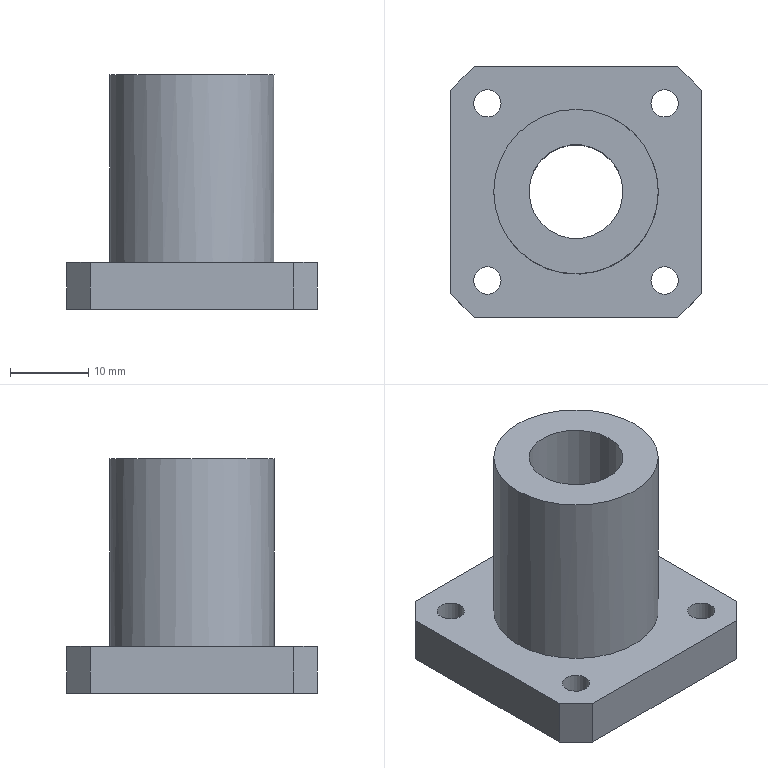Part | STEP file | 冲床-300配套压波_id778_x_t | 1 solid | 25 faces | box 32 x 32 x 30 mm | volume 10494 mm3 | plane 15 | cylinder 10 | commonest cylinder face diameters 3.5 x4 6 x4 12 x1 21 x1
STEP:
#1=CARTESIAN_POINT('',(1749.5,-85.,108.));
#2=VERTEX_POINT('',#1);
#3=CARTESIAN_POINT('',(1760.,-85.,108.));
#4=DIRECTION('',(0.,0.,1.));
#5=DIRECTION('',(-1.,0.,0.));
#6=AXIS2_PLACEMENT_3D('',#3,#4,#5);
#7=CIRCLE('',#6,10.5);
#8=EDGE_CURVE('',#2,#2,#7,.T.);
#9=ORIENTED_EDGE('',*,*,#8,.T.);
#10=EDGE_LOOP('',(#9));
#11=FACE_BOUND('',#10,.T.);
#12=CARTESIAN_POINT('',(1770.5,-85.,132.));
#13=VERTEX_POINT('',#12);
#14=CARTESIAN_POINT('',(1760.,-85.,132.));
#15=DIRECTION('',(0.,0.,1.));
#16=DIRECTION('',(1.,0.,0.));
#17=AXIS2_PLACEMENT_3D('',#14,#15,#16);
#18=CIRCLE('',#17,10.5);
#19=EDGE_CURVE('',#13,#13,#18,.T.);
#20=ORIENTED_EDGE('',*,*,#19,.F.);
#21=EDGE_LOOP('',(#20));
#22=FACE_BOUND('',#21,.T.);
#23=CARTESIAN_POINT('',(1760.,-85.,132.));
#24=DIRECTION('',(0.,0.,-1.));
#25=DIRECTION('',(-1.,0.,0.));
#26=AXIS2_PLACEMENT_3D('',#23,#24,#25);
#27=CYLINDRICAL_SURFACE('',#26,10.5);
#28=ADVANCED_FACE('',(#11,#22),#27,.T.);
#29=CARTESIAN_POINT('',(1754.,-85.,102.));
#30=VERTEX_POINT('',#29);
#31=CARTESIAN_POINT('',(1760.,-85.,102.));
#32=DIRECTION('',(0.,0.,-1.));
#33=DIRECTION('',(-1.,0.,0.));
#34=AXIS2_PLACEMENT_3D('',#31,#32,#33);
#35=CIRCLE('',#34,6.);
#36=EDGE_CURVE('',#30,#30,#35,.T.);
#37=ORIENTED_EDGE('',*,*,#36,.T.);
#38=EDGE_LOOP('',(#37));
#39=FACE_BOUND('',#38,.T.);
#40=CARTESIAN_POINT('',(1766.,-85.,132.));
#41=VERTEX_POINT('',#40);
#42=CARTESIAN_POINT('',(1760.,-85.,132.));
#43=DIRECTION('',(0.,0.,-1.));
#44=DIRECTION('',(1.,0.,0.));
#45=AXIS2_PLACEMENT_3D('',#42,#43,#44);
#46=CIRCLE('',#45,6.);
#47=EDGE_CURVE('',#41,#41,#46,.T.);
#48=ORIENTED_EDGE('',*,*,#47,.F.);
#49=EDGE_LOOP('',(#48));
#50=FACE_BOUND('',#49,.T.);
#51=CARTESIAN_POINT('',(1760.,-85.,72.));
#52=DIRECTION('',(0.,0.,1.));
#53=DIRECTION('',(1.,0.,0.));
#54=AXIS2_PLACEMENT_3D('',#51,#52,#53);
#55=CYLINDRICAL_SURFACE('',#54,6.);
#56=ADVANCED_FACE('',(#39,#50),#55,.F.);
#57=ORIENTED_EDGE('',*,*,#36,.F.);
#58=EDGE_LOOP('',(#57));
#59=FACE_BOUND('',#58,.T.);
#60=CARTESIAN_POINT('',(1768.314,-96.314,102.));
#61=VERTEX_POINT('',#60);
#62=CARTESIAN_POINT('',(1771.314,-96.314,102.));
#63=DIRECTION('',(0.,0.,-1.));
#64=DIRECTION('',(-1.,0.,0.));
#65=AXIS2_PLACEMENT_3D('',#62,#63,#64);
#66=CIRCLE('',#65,3.);
#67=EDGE_CURVE('',#61,#61,#66,.T.);
#68=ORIENTED_EDGE('',*,*,#67,.F.);
#69=EDGE_LOOP('',(#68));
#70=FACE_BOUND('',#69,.T.);
#71=CARTESIAN_POINT('',(1745.686,-73.686,102.));
#72=VERTEX_POINT('',#71);
#73=CARTESIAN_POINT('',(1748.686,-73.686,102.));
#74=DIRECTION('',(0.,0.,-1.));
#75=DIRECTION('',(-1.,0.,0.));
#76=AXIS2_PLACEMENT_3D('',#73,#74,#75);
#77=CIRCLE('',#76,3.);
#78=EDGE_CURVE('',#72,#72,#77,.T.);
#79=ORIENTED_EDGE('',*,*,#78,.F.);
#80=EDGE_LOOP('',(#79));
#81=FACE_BOUND('',#80,.T.);
#82=CARTESIAN_POINT('',(1773.,-101.,102.));
#83=VERTEX_POINT('',#82);
#84=CARTESIAN_POINT('',(1747.,-101.,102.));
#85=VERTEX_POINT('',#84);
#86=CARTESIAN_POINT('',(1744.,-101.,102.));
#87=DIRECTION('',(-1.,0.,0.));
#88=VECTOR('',#87,1.);
#89=LINE('',#86,#88);
#90=EDGE_CURVE('',#83,#85,#89,.T.);
#91=ORIENTED_EDGE('',*,*,#90,.T.);
#92=CARTESIAN_POINT('',(1744.,-98.,102.));
#93=VERTEX_POINT('',#92);
#94=CARTESIAN_POINT('',(1745.5,-99.5,102.));
#95=DIRECTION('',(-0.7071,0.7071,0.));
#96=VECTOR('',#95,1.);
#97=LINE('',#94,#96);
#98=EDGE_CURVE('',#85,#93,#97,.T.);
#99=ORIENTED_EDGE('',*,*,#98,.T.);
#100=CARTESIAN_POINT('',(1744.,-72.,102.));
#101=VERTEX_POINT('',#100);
#102=CARTESIAN_POINT('',(1744.,-69.,102.));
#103=DIRECTION('',(0.,1.,0.));
#104=VECTOR('',#103,1.);
#105=LINE('',#102,#104);
#106=EDGE_CURVE('',#93,#101,#105,.T.);
#107=ORIENTED_EDGE('',*,*,#106,.T.);
#108=CARTESIAN_POINT('',(1747.,-69.,102.));
#109=VERTEX_POINT('',#108);
#110=CARTESIAN_POINT('',(1756.814,-59.186,102.));
#111=DIRECTION('',(0.7071,0.7071,0.));
#112=VECTOR('',#111,1.);
#113=LINE('',#110,#112);
#114=EDGE_CURVE('',#101,#109,#113,.T.);
#115=ORIENTED_EDGE('',*,*,#114,.T.);
#116=CARTESIAN_POINT('',(1773.,-69.,102.));
#117=VERTEX_POINT('',#116);
#118=CARTESIAN_POINT('',(1776.,-69.,102.));
#119=DIRECTION('',(1.,0.,0.));
#120=VECTOR('',#119,1.);
#121=LINE('',#118,#120);
#122=EDGE_CURVE('',#109,#117,#121,.T.);
#123=ORIENTED_EDGE('',*,*,#122,.T.);
#124=CARTESIAN_POINT('',(1776.,-72.,102.));
#125=VERTEX_POINT('',#124);
#126=CARTESIAN_POINT('',(1774.5,-70.5,102.));
#127=DIRECTION('',(0.7071,-0.7071,0.));
#128=VECTOR('',#127,1.);
#129=LINE('',#126,#128);
#130=EDGE_CURVE('',#117,#125,#129,.T.);
#131=ORIENTED_EDGE('',*,*,#130,.T.);
#132=CARTESIAN_POINT('',(1776.,-98.,102.));
#133=VERTEX_POINT('',#132);
#134=CARTESIAN_POINT('',(1776.,-101.,102.));
#135=DIRECTION('',(0.,-1.,0.));
#136=VECTOR('',#135,1.);
#137=LINE('',#134,#136);
#138=EDGE_CURVE('',#125,#133,#137,.T.);
#139=ORIENTED_EDGE('',*,*,#138,.T.);
#140=CARTESIAN_POINT('',(1785.814,-88.186,102.));
#141=DIRECTION('',(-0.7071,-0.7071,0.));
#142=VECTOR('',#141,1.);
#143=LINE('',#140,#142);
#144=EDGE_CURVE('',#133,#83,#143,.T.);
#145=ORIENTED_EDGE('',*,*,#144,.T.);
#146=EDGE_LOOP('',(#91,#99,#107,#115,#123,#131,#139,#145));
#147=FACE_BOUND('',#146,.T.);
#148=CARTESIAN_POINT('',(1768.314,-73.686,102.));
#149=VERTEX_POINT('',#148);
#150=CARTESIAN_POINT('',(1771.314,-73.686,102.));
#151=DIRECTION('',(0.,0.,-1.));
#152=DIRECTION('',(-1.,0.,0.));
#153=AXIS2_PLACEMENT_3D('',#150,#151,#152);
#154=CIRCLE('',#153,3.);
#155=EDGE_CURVE('',#149,#149,#154,.T.);
#156=ORIENTED_EDGE('',*,*,#155,.F.);
#157=EDGE_LOOP('',(#156));
#158=FACE_BOUND('',#157,.T.);
#159=CARTESIAN_POINT('',(1745.686,-96.314,102.));
#160=VERTEX_POINT('',#159);
#161=CARTESIAN_POINT('',(1748.686,-96.314,102.));
#162=DIRECTION('',(0.,0.,1.));
#163=DIRECTION('',(-1.,0.,0.));
#164=AXIS2_PLACEMENT_3D('',#161,#162,#163);
#165=CIRCLE('',#164,3.);
#166=EDGE_CURVE('',#160,#160,#165,.T.);
#167=ORIENTED_EDGE('',*,*,#166,.T.);
#168=EDGE_LOOP('',(#167));
#169=FACE_BOUND('',#168,.T.);
#170=CARTESIAN_POINT('',(1771.314,-73.686,102.));
#171=DIRECTION('',(0.,0.,-1.));
#172=DIRECTION('',(-1.,0.,0.));
#173=AXIS2_PLACEMENT_3D('',#170,#171,#172);
#174=PLANE('',#173);
#175=ADVANCED_FACE('',(#59,#70,#81,#147,#158,#169),#174,.T.);
#176=CARTESIAN_POINT('',(1746.936,-73.686,108.));
#177=VERTEX_POINT('',#176);
#178=CARTESIAN_POINT('',(1748.686,-73.686,108.));
#179=DIRECTION('',(0.,0.,-1.));
#180=DIRECTION('',(-1.,0.,0.));
#181=AXIS2_PLACEMENT_3D('',#178,#179,#180);
#182=CIRCLE('',#181,1.75);
#183=EDGE_CURVE('',#177,#177,#182,.T.);
#184=ORIENTED_EDGE('',*,*,#183,.F.);
#185=EDGE_LOOP('',(#184));
#186=FACE_BOUND('',#185,.T.);
#187=CARTESIAN_POINT('',(1746.936,-73.686,105.1));
#188=VERTEX_POINT('',#187);
#189=CARTESIAN_POINT('',(1748.686,-73.686,105.1));
#190=DIRECTION('',(0.,0.,-1.));
#191=DIRECTION('',(-1.,0.,0.));
#192=AXIS2_PLACEMENT_3D('',#189,#190,#191);
#193=CIRCLE('',#192,1.75);
#194=EDGE_CURVE('',#188,#188,#193,.T.);
#195=ORIENTED_EDGE('',*,*,#194,.T.);
#196=EDGE_LOOP('',(#195));
#197=FACE_BOUND('',#196,.T.);
#198=CARTESIAN_POINT('',(1748.686,-73.686,102.));
#199=DIRECTION('',(0.,0.,1.));
#200=DIRECTION('',(1.,0.,0.));
#201=AXIS2_PLACEMENT_3D('',#198,#199,#200);
#202=CYLINDRICAL_SURFACE('',#201,1.75);
#203=ADVANCED_FACE('',(#186,#197),#202,.F.);
#204=CARTESIAN_POINT('',(1769.564,-96.314,108.));
#205=VERTEX_POINT('',#204);
#206=CARTESIAN_POINT('',(1771.314,-96.314,108.));
#207=DIRECTION('',(0.,0.,-1.));
#208=DIRECTION('',(-1.,0.,0.));
#209=AXIS2_PLACEMENT_3D('',#206,#207,#208);
#210=CIRCLE('',#209,1.75);
#211=EDGE_CURVE('',#205,#205,#210,.T.);
#212=ORIENTED_EDGE('',*,*,#211,.F.);
#213=EDGE_LOOP('',(#212));
#214=FACE_BOUND('',#213,.T.);
#215=CARTESIAN_POINT('',(1769.564,-96.314,105.1));
#216=VERTEX_POINT('',#215);
#217=CARTESIAN_POINT('',(1771.314,-96.314,105.1));
#218=DIRECTION('',(0.,0.,-1.));
#219=DIRECTION('',(-1.,0.,0.));
#220=AXIS2_PLACEMENT_3D('',#217,#218,#219);
#221=CIRCLE('',#220,1.75);
#222=EDGE_CURVE('',#216,#216,#221,.T.);
#223=ORIENTED_EDGE('',*,*,#222,.T.);
#224=EDGE_LOOP('',(#223));
#225=FACE_BOUND('',#224,.T.);
#226=CARTESIAN_POINT('',(1771.314,-96.314,102.));
#227=DIRECTION('',(0.,0.,1.));
#228=DIRECTION('',(1.,0.,0.));
#229=AXIS2_PLACEMENT_3D('',#226,#227,#228);
#230=CYLINDRICAL_SURFACE('',#229,1.75);
#231=ADVANCED_FACE('',(#214,#225),#230,.F.);
#232=CARTESIAN_POINT('',(1769.564,-73.686,108.));
#233=VERTEX_POINT('',#232);
#234=CARTESIAN_POINT('',(1771.314,-73.686,108.));
#235=DIRECTION('',(0.,0.,-1.));
#236=DIRECTION('',(-1.,0.,0.));
#237=AXIS2_PLACEMENT_3D('',#234,#235,#236);
#238=CIRCLE('',#237,1.75);
#239=EDGE_CURVE('',#233,#233,#238,.T.);
#240=ORIENTED_EDGE('',*,*,#239,.F.);
#241=EDGE_LOOP('',(#240));
#242=FACE_BOUND('',#241,.T.);
#243=CARTESIAN_POINT('',(1769.564,-73.686,105.1));
#244=VERTEX_POINT('',#243);
#245=CARTESIAN_POINT('',(1771.314,-73.686,105.1));
#246=DIRECTION('',(0.,0.,-1.));
#247=DIRECTION('',(-1.,0.,0.));
#248=AXIS2_PLACEMENT_3D('',#245,#246,#247);
#249=CIRCLE('',#248,1.75);
#250=EDGE_CURVE('',#244,#244,#249,.T.);
#251=ORIENTED_EDGE('',*,*,#250,.T.);
#252=EDGE_LOOP('',(#251));
#253=FACE_BOUND('',#252,.T.);
#254=CARTESIAN_POINT('',(1771.314,-73.686,102.));
#255=DIRECTION('',(0.,0.,1.));
#256=DIRECTION('',(1.,0.,0.));
#257=AXIS2_PLACEMENT_3D('',#254,#255,#256);
#258=CYLINDRICAL_SURFACE('',#257,1.75);
#259=ADVANCED_FACE('',(#242,#253),#258,.F.);
#260=ORIENTED_EDGE('',*,*,#138,.F.);
#261=CARTESIAN_POINT('',(1776.,-72.,108.));
#262=VERTEX_POINT('',#261);
#263=CARTESIAN_POINT('',(1776.,-72.,102.));
#264=DIRECTION('',(0.,0.,1.));
#265=VECTOR('',#264,1.);
#266=LINE('',#263,#265);
#267=EDGE_CURVE('',#125,#262,#266,.T.);
#268=ORIENTED_EDGE('',*,*,#267,.T.);
#269=CARTESIAN_POINT('',(1776.,-98.,108.));
#270=VERTEX_POINT('',#269);
#271=CARTESIAN_POINT('',(1776.,-101.,108.));
#272=DIRECTION('',(0.,-1.,0.));
#273=VECTOR('',#272,1.);
#274=LINE('',#271,#273);
#275=EDGE_CURVE('',#262,#270,#274,.T.);
#276=ORIENTED_EDGE('',*,*,#275,.T.);
#277=CARTESIAN_POINT('',(1776.,-98.,102.));
#278=DIRECTION('',(0.,0.,-1.));
#279=VECTOR('',#278,1.);
#280=LINE('',#277,#279);
#281=EDGE_CURVE('',#270,#133,#280,.T.);
#282=ORIENTED_EDGE('',*,*,#281,.T.);
#283=EDGE_LOOP('',(#260,#268,#276,#282));
#284=FACE_OUTER_BOUND('',#283,.T.);
#285=CARTESIAN_POINT('',(1776.,-101.,102.));
#286=DIRECTION('',(-1.,0.,0.));
#287=DIRECTION('',(0.,0.,1.));
#288=AXIS2_PLACEMENT_3D('',#285,#286,#287);
#289=PLANE('',#288);
#290=ADVANCED_FACE('',(#284),#289,.F.);
#291=ORIENTED_EDGE('',*,*,#122,.F.);
#292=CARTESIAN_POINT('',(1747.,-69.,108.));
#293=VERTEX_POINT('',#292);
#294=CARTESIAN_POINT('',(1747.,-69.,102.));
#295=DIRECTION('',(0.,0.,1.));
#296=VECTOR('',#295,1.);
#297=LINE('',#294,#296);
#298=EDGE_CURVE('',#109,#293,#297,.T.);
#299=ORIENTED_EDGE('',*,*,#298,.T.);
#300=CARTESIAN_POINT('',(1773.,-69.,108.));
#301=VERTEX_POINT('',#300);
#302=CARTESIAN_POINT('',(1776.,-69.,108.));
#303=DIRECTION('',(1.,0.,0.));
#304=VECTOR('',#303,1.);
#305=LINE('',#302,#304);
#306=EDGE_CURVE('',#293,#301,#305,.T.);
#307=ORIENTED_EDGE('',*,*,#306,.T.);
#308=CARTESIAN_POINT('',(1773.,-69.,102.));
#309=DIRECTION('',(0.,0.,-1.));
#310=VECTOR('',#309,1.);
#311=LINE('',#308,#310);
#312=EDGE_CURVE('',#301,#117,#311,.T.);
#313=ORIENTED_EDGE('',*,*,#312,.T.);
#314=EDGE_LOOP('',(#291,#299,#307,#313));
#315=FACE_OUTER_BOUND('',#314,.T.);
#316=CARTESIAN_POINT('',(1776.,-69.,102.));
#317=DIRECTION('',(0.,-1.,0.));
#318=DIRECTION('',(0.,0.,-1.));
#319=AXIS2_PLACEMENT_3D('',#316,#317,#318);
#320=PLANE('',#319);
#321=ADVANCED_FACE('',(#315),#320,.F.);
#322=CARTESIAN_POINT('',(1744.,-98.,108.));
#323=VERTEX_POINT('',#322);
#324=CARTESIAN_POINT('',(1744.,-72.,108.));
#325=VERTEX_POINT('',#324);
#326=CARTESIAN_POINT('',(1744.,-69.,108.));
#327=DIRECTION('',(0.,1.,0.));
#328=VECTOR('',#327,1.);
#329=LINE('',#326,#328);
#330=EDGE_CURVE('',#323,#325,#329,.T.);
#331=ORIENTED_EDGE('',*,*,#330,.T.);
#332=CARTESIAN_POINT('',(1744.,-72.,102.));
#333=DIRECTION('',(0.,0.,-1.));
#334=VECTOR('',#333,1.);
#335=LINE('',#332,#334);
#336=EDGE_CURVE('',#325,#101,#335,.T.);
#337=ORIENTED_EDGE('',*,*,#336,.T.);
#338=ORIENTED_EDGE('',*,*,#106,.F.);
#339=CARTESIAN_POINT('',(1744.,-98.,102.));
#340=DIRECTION('',(0.,0.,1.));
#341=VECTOR('',#340,1.);
#342=LINE('',#339,#341);
#343=EDGE_CURVE('',#93,#323,#342,.T.);
#344=ORIENTED_EDGE('',*,*,#343,.T.);
#345=EDGE_LOOP('',(#331,#337,#338,#344));
#346=FACE_OUTER_BOUND('',#345,.T.);
#347=CARTESIAN_POINT('',(1744.,-69.,102.));
#348=DIRECTION('',(1.,0.,0.));
#349=DIRECTION('',(0.,0.,-1.));
#350=AXIS2_PLACEMENT_3D('',#347,#348,#349);
#351=PLANE('',#350);
#352=ADVANCED_FACE('',(#346),#351,.F.);
#353=CARTESIAN_POINT('',(1773.,-101.,108.));
#354=VERTEX_POINT('',#353);
#355=CARTESIAN_POINT('',(1747.,-101.,108.));
#356=VERTEX_POINT('',#355);
#357=CARTESIAN_POINT('',(1744.,-101.,108.));
#358=DIRECTION('',(-1.,0.,0.));
#359=VECTOR('',#358,1.);
#360=LINE('',#357,#359);
#361=EDGE_CURVE('',#354,#356,#360,.T.);
#362=ORIENTED_EDGE('',*,*,#361,.T.);
#363=CARTESIAN_POINT('',(1747.,-101.,102.));
#364=DIRECTION('',(0.,0.,-1.));
#365=VECTOR('',#364,1.);
#366=LINE('',#363,#365);
#367=EDGE_CURVE('',#356,#85,#366,.T.);
#368=ORIENTED_EDGE('',*,*,#367,.T.);
#369=ORIENTED_EDGE('',*,*,#90,.F.);
#370=CARTESIAN_POINT('',(1773.,-101.,102.));
#371=DIRECTION('',(0.,0.,1.));
#372=VECTOR('',#371,1.);
#373=LINE('',#370,#372);
#374=EDGE_CURVE('',#83,#354,#373,.T.);
#375=ORIENTED_EDGE('',*,*,#374,.T.);
#376=EDGE_LOOP('',(#362,#368,#369,#375));
#377=FACE_OUTER_BOUND('',#376,.T.);
#378=CARTESIAN_POINT('',(1744.,-101.,102.));
#379=DIRECTION('',(0.,1.,0.));
#380=DIRECTION('',(0.,0.,1.));
#381=AXIS2_PLACEMENT_3D('',#378,#379,#380);
#382=PLANE('',#381);
#383=ADVANCED_FACE('',(#377),#382,.F.);
#384=CARTESIAN_POINT('',(1746.936,-96.314,105.1));
#385=VERTEX_POINT('',#384);
#386=CARTESIAN_POINT('',(1748.686,-96.314,105.1));
#387=DIRECTION('',(0.,0.,1.));
#388=DIRECTION('',(-1.,0.,0.));
#389=AXIS2_PLACEMENT_3D('',#386,#387,#388);
#390=CIRCLE('',#389,1.75);
#391=EDGE_CURVE('',#385,#385,#390,.T.);
#392=ORIENTED_EDGE('',*,*,#391,.F.);
#393=EDGE_LOOP('',(#392));
#394=FACE_BOUND('',#393,.T.);
#395=CARTESIAN_POINT('',(1746.936,-96.314,108.));
#396=VERTEX_POINT('',#395);
#397=CARTESIAN_POINT('',(1748.686,-96.314,108.));
#398=DIRECTION('',(0.,0.,-1.));
#399=DIRECTION('',(-1.,0.,0.));
#400=AXIS2_PLACEMENT_3D('',#397,#398,#399);
#401=CIRCLE('',#400,1.75);
#402=EDGE_CURVE('',#396,#396,#401,.T.);
#403=ORIENTED_EDGE('',*,*,#402,.F.);
#404=EDGE_LOOP('',(#403));
#405=FACE_BOUND('',#404,.T.);
#406=CARTESIAN_POINT('',(1748.686,-96.314,102.));
#407=DIRECTION('',(0.,0.,1.));
#408=DIRECTION('',(1.,0.,0.));
#409=AXIS2_PLACEMENT_3D('',#406,#407,#408);
#410=CYLINDRICAL_SURFACE('',#409,1.75);
#411=ADVANCED_FACE('',(#394,#405),#410,.F.);
#412=ORIENTED_EDGE('',*,*,#8,.F.);
#413=EDGE_LOOP('',(#412));
#414=FACE_BOUND('',#413,.T.);
#415=ORIENTED_EDGE('',*,*,#275,.F.);
#416=CARTESIAN_POINT('',(1773.,-69.,108.));
#417=DIRECTION('',(-0.7071,0.7071,0.));
#418=VECTOR('',#417,1.);
#419=LINE('',#416,#418);
#420=EDGE_CURVE('',#262,#301,#419,.T.);
#421=ORIENTED_EDGE('',*,*,#420,.T.);
#422=ORIENTED_EDGE('',*,*,#306,.F.);
#423=CARTESIAN_POINT('',(1744.,-72.,108.));
#424=DIRECTION('',(-0.7071,-0.7071,0.));
#425=VECTOR('',#424,1.);
#426=LINE('',#423,#425);
#427=EDGE_CURVE('',#293,#325,#426,.T.);
#428=ORIENTED_EDGE('',*,*,#427,.T.);
#429=ORIENTED_EDGE('',*,*,#330,.F.);
#430=CARTESIAN_POINT('',(1747.,-101.,108.));
#431=DIRECTION('',(0.7071,-0.7071,0.));
#432=VECTOR('',#431,1.);
#433=LINE('',#430,#432);
#434=EDGE_CURVE('',#323,#356,#433,.T.);
#435=ORIENTED_EDGE('',*,*,#434,.T.);
#436=ORIENTED_EDGE('',*,*,#361,.F.);
#437=CARTESIAN_POINT('',(1776.,-98.,108.));
#438=DIRECTION('',(0.7071,0.7071,0.));
#439=VECTOR('',#438,1.);
#440=LINE('',#437,#439);
#441=EDGE_CURVE('',#354,#270,#440,.T.);
#442=ORIENTED_EDGE('',*,*,#441,.T.);
#443=EDGE_LOOP('',(#415,#421,#422,#428,#429,#435,#436,#442));
#444=FACE_BOUND('',#443,.T.);
#445=ORIENTED_EDGE('',*,*,#239,.T.);
#446=EDGE_LOOP('',(#445));
#447=FACE_BOUND('',#446,.T.);
#448=ORIENTED_EDGE('',*,*,#211,.T.);
#449=EDGE_LOOP('',(#448));
#450=FACE_BOUND('',#449,.T.);
#451=ORIENTED_EDGE('',*,*,#183,.T.);
#452=EDGE_LOOP('',(#451));
#453=FACE_BOUND('',#452,.T.);
#454=ORIENTED_EDGE('',*,*,#402,.T.);
#455=EDGE_LOOP('',(#454));
#456=FACE_BOUND('',#455,.T.);
#457=CARTESIAN_POINT('',(1771.314,-73.686,108.));
#458=DIRECTION('',(0.,0.,-1.));
#459=DIRECTION('',(-1.,0.,0.));
#460=AXIS2_PLACEMENT_3D('',#457,#458,#459);
#461=PLANE('',#460);
#462=ADVANCED_FACE('',(#414,#444,#447,#450,#453,#456),#461,.F.);
#463=CARTESIAN_POINT('',(1745.686,-96.314,105.1));
#464=VERTEX_POINT('',#463);
#465=CARTESIAN_POINT('',(1748.686,-96.314,105.1));
#466=DIRECTION('',(0.,0.,-1.));
#467=DIRECTION('',(-1.,0.,0.));
#468=AXIS2_PLACEMENT_3D('',#465,#466,#467);
#469=CIRCLE('',#468,3.);
#470=EDGE_CURVE('',#464,#464,#469,.T.);
#471=ORIENTED_EDGE('',*,*,#470,.F.);
#472=EDGE_LOOP('',(#471));
#473=FACE_BOUND('',#472,.T.);
#474=ORIENTED_EDGE('',*,*,#166,.F.);
#475=EDGE_LOOP('',(#474));
#476=FACE_BOUND('',#475,.T.);
#477=CARTESIAN_POINT('',(1748.686,-96.314,105.1));
#478=DIRECTION('',(0.,0.,-1.));
#479=DIRECTION('',(-1.,0.,0.));
#480=AXIS2_PLACEMENT_3D('',#477,#478,#479);
#481=CYLINDRICAL_SURFACE('',#480,3.);
#482=ADVANCED_FACE('',(#473,#476),#481,.F.);
#483=ORIENTED_EDGE('',*,*,#391,.T.);
#484=EDGE_LOOP('',(#483));
#485=FACE_BOUND('',#484,.T.);
#486=ORIENTED_EDGE('',*,*,#470,.T.);
#487=EDGE_LOOP('',(#486));
#488=FACE_BOUND('',#487,.T.);
#489=CARTESIAN_POINT('',(1771.314,-73.686,105.1));
#490=DIRECTION('',(0.,0.,-1.));
#491=DIRECTION('',(-1.,0.,0.));
#492=AXIS2_PLACEMENT_3D('',#489,#490,#491);
#493=PLANE('',#492);
#494=ADVANCED_FACE('',(#485,#488),#493,.T.);
#495=CARTESIAN_POINT('',(1768.314,-73.686,105.1));
#496=VERTEX_POINT('',#495);
#497=CARTESIAN_POINT('',(1771.314,-73.686,105.1));
#498=DIRECTION('',(0.,0.,1.));
#499=DIRECTION('',(-1.,0.,0.));
#500=AXIS2_PLACEMENT_3D('',#497,#498,#499);
#501=CIRCLE('',#500,3.);
#502=EDGE_CURVE('',#496,#496,#501,.T.);
#503=ORIENTED_EDGE('',*,*,#502,.T.);
#504=EDGE_LOOP('',(#503));
#505=FACE_BOUND('',#504,.T.);
#506=ORIENTED_EDGE('',*,*,#155,.T.);
#507=EDGE_LOOP('',(#506));
#508=FACE_BOUND('',#507,.T.);
#509=CARTESIAN_POINT('',(1771.314,-73.686,105.1));
#510=DIRECTION('',(0.,0.,-1.));
#511=DIRECTION('',(-1.,0.,0.));
#512=AXIS2_PLACEMENT_3D('',#509,#510,#511);
#513=CYLINDRICAL_SURFACE('',#512,3.);
#514=ADVANCED_FACE('',(#505,#508),#513,.F.);
#515=ORIENTED_EDGE('',*,*,#250,.F.);
#516=EDGE_LOOP('',(#515));
#517=FACE_BOUND('',#516,.T.);
#518=ORIENTED_EDGE('',*,*,#502,.F.);
#519=EDGE_LOOP('',(#518));
#520=FACE_BOUND('',#519,.T.);
#521=CARTESIAN_POINT('',(1771.314,-73.686,105.1));
#522=DIRECTION('',(0.,0.,-1.));
#523=DIRECTION('',(-1.,0.,0.));
#524=AXIS2_PLACEMENT_3D('',#521,#522,#523);
#525=PLANE('',#524);
#526=ADVANCED_FACE('',(#517,#520),#525,.T.);
#527=CARTESIAN_POINT('',(1768.314,-96.314,105.1));
#528=VERTEX_POINT('',#527);
#529=CARTESIAN_POINT('',(1771.314,-96.314,105.1));
#530=DIRECTION('',(0.,0.,1.));
#531=DIRECTION('',(-1.,0.,0.));
#532=AXIS2_PLACEMENT_3D('',#529,#530,#531);
#533=CIRCLE('',#532,3.);
#534=EDGE_CURVE('',#528,#528,#533,.T.);
#535=ORIENTED_EDGE('',*,*,#534,.T.);
#536=EDGE_LOOP('',(#535));
#537=FACE_BOUND('',#536,.T.);
#538=ORIENTED_EDGE('',*,*,#67,.T.);
#539=EDGE_LOOP('',(#538));
#540=FACE_BOUND('',#539,.T.);
#541=CARTESIAN_POINT('',(1771.314,-96.314,105.1));
#542=DIRECTION('',(0.,0.,-1.));
#543=DIRECTION('',(-1.,0.,0.));
#544=AXIS2_PLACEMENT_3D('',#541,#542,#543);
#545=CYLINDRICAL_SURFACE('',#544,3.);
#546=ADVANCED_FACE('',(#537,#540),#545,.F.);
#547=ORIENTED_EDGE('',*,*,#222,.F.);
#548=EDGE_LOOP('',(#547));
#549=FACE_BOUND('',#548,.T.);
#550=ORIENTED_EDGE('',*,*,#534,.F.);
#551=EDGE_LOOP('',(#550));
#552=FACE_BOUND('',#551,.T.);
#553=CARTESIAN_POINT('',(1771.314,-73.686,105.1));
#554=DIRECTION('',(0.,0.,-1.));
#555=DIRECTION('',(-1.,0.,0.));
#556=AXIS2_PLACEMENT_3D('',#553,#554,#555);
#557=PLANE('',#556);
#558=ADVANCED_FACE('',(#549,#552),#557,.T.);
#559=CARTESIAN_POINT('',(1745.686,-73.686,105.1));
#560=VERTEX_POINT('',#559);
#561=CARTESIAN_POINT('',(1748.686,-73.686,105.1));
#562=DIRECTION('',(0.,0.,1.));
#563=DIRECTION('',(-1.,0.,0.));
#564=AXIS2_PLACEMENT_3D('',#561,#562,#563);
#565=CIRCLE('',#564,3.);
#566=EDGE_CURVE('',#560,#560,#565,.T.);
#567=ORIENTED_EDGE('',*,*,#566,.T.);
#568=EDGE_LOOP('',(#567));
#569=FACE_BOUND('',#568,.T.);
#570=ORIENTED_EDGE('',*,*,#78,.T.);
#571=EDGE_LOOP('',(#570));
#572=FACE_BOUND('',#571,.T.);
#573=CARTESIAN_POINT('',(1748.686,-73.686,105.1));
#574=DIRECTION('',(0.,0.,-1.));
#575=DIRECTION('',(-1.,0.,0.));
#576=AXIS2_PLACEMENT_3D('',#573,#574,#575);
#577=CYLINDRICAL_SURFACE('',#576,3.);
#578=ADVANCED_FACE('',(#569,#572),#577,.F.);
#579=ORIENTED_EDGE('',*,*,#194,.F.);
#580=EDGE_LOOP('',(#579));
#581=FACE_BOUND('',#580,.T.);
#582=ORIENTED_EDGE('',*,*,#566,.F.);
#583=EDGE_LOOP('',(#582));
#584=FACE_BOUND('',#583,.T.);
#585=CARTESIAN_POINT('',(1771.314,-73.686,105.1));
#586=DIRECTION('',(0.,0.,-1.));
#587=DIRECTION('',(-1.,0.,0.));
#588=AXIS2_PLACEMENT_3D('',#585,#586,#587);
#589=PLANE('',#588);
#590=ADVANCED_FACE('',(#581,#584),#589,.T.);
#591=ORIENTED_EDGE('',*,*,#144,.F.);
#592=ORIENTED_EDGE('',*,*,#281,.F.);
#593=ORIENTED_EDGE('',*,*,#441,.F.);
#594=ORIENTED_EDGE('',*,*,#374,.F.);
#595=EDGE_LOOP('',(#591,#592,#593,#594));
#596=FACE_OUTER_BOUND('',#595,.T.);
#597=CARTESIAN_POINT('',(1776.,-98.,102.));
#598=DIRECTION('',(-0.7071,0.7071,0.));
#599=DIRECTION('',(0.,0.,1.));
#600=AXIS2_PLACEMENT_3D('',#597,#598,#599);
#601=PLANE('',#600);
#602=ADVANCED_FACE('',(#596),#601,.F.);
#603=ORIENTED_EDGE('',*,*,#98,.F.);
#604=ORIENTED_EDGE('',*,*,#367,.F.);
#605=ORIENTED_EDGE('',*,*,#434,.F.);
#606=ORIENTED_EDGE('',*,*,#343,.F.);
#607=EDGE_LOOP('',(#603,#604,#605,#606));
#608=FACE_OUTER_BOUND('',#607,.T.);
#609=CARTESIAN_POINT('',(1747.,-101.,102.));
#610=DIRECTION('',(0.7071,0.7071,0.));
#611=DIRECTION('',(0.,0.,1.));
#612=AXIS2_PLACEMENT_3D('',#609,#610,#611);
#613=PLANE('',#612);
#614=ADVANCED_FACE('',(#608),#613,.F.);
#615=ORIENTED_EDGE('',*,*,#130,.F.);
#616=ORIENTED_EDGE('',*,*,#312,.F.);
#617=ORIENTED_EDGE('',*,*,#420,.F.);
#618=ORIENTED_EDGE('',*,*,#267,.F.);
#619=EDGE_LOOP('',(#615,#616,#617,#618));
#620=FACE_OUTER_BOUND('',#619,.T.);
#621=CARTESIAN_POINT('',(1773.,-69.,102.));
#622=DIRECTION('',(-0.7071,-0.7071,0.));
#623=DIRECTION('',(0.,0.,1.));
#624=AXIS2_PLACEMENT_3D('',#621,#622,#623);
#625=PLANE('',#624);
#626=ADVANCED_FACE('',(#620),#625,.F.);
#627=ORIENTED_EDGE('',*,*,#114,.F.);
#628=ORIENTED_EDGE('',*,*,#336,.F.);
#629=ORIENTED_EDGE('',*,*,#427,.F.);
#630=ORIENTED_EDGE('',*,*,#298,.F.);
#631=EDGE_LOOP('',(#627,#628,#629,#630));
#632=FACE_OUTER_BOUND('',#631,.T.);
#633=CARTESIAN_POINT('',(1744.,-72.,102.));
#634=DIRECTION('',(0.7071,-0.7071,0.));
#635=DIRECTION('',(0.,0.,1.));
#636=AXIS2_PLACEMENT_3D('',#633,#634,#635);
#637=PLANE('',#636);
#638=ADVANCED_FACE('',(#632),#637,.F.);
#639=ORIENTED_EDGE('',*,*,#47,.T.);
#640=EDGE_LOOP('',(#639));
#641=FACE_BOUND('',#640,.T.);
#642=ORIENTED_EDGE('',*,*,#19,.T.);
#643=EDGE_LOOP('',(#642));
#644=FACE_BOUND('',#643,.T.);
#645=CARTESIAN_POINT('',(1760.,-85.,132.));
#646=DIRECTION('',(0.,0.,1.));
#647=DIRECTION('',(1.,0.,0.));
#648=AXIS2_PLACEMENT_3D('',#645,#646,#647);
#649=PLANE('',#648);
#650=ADVANCED_FACE('',(#641,#644),#649,.T.);
#651=CLOSED_SHELL('',(#28,#56,#175,#203,#231,#259,#290,#321,#352,#383,#411,#462,#482,#494,#514,#526,#546,#558,#578,#590,#602,#614,#626,#638,#650));
#652=MANIFOLD_SOLID_BREP('',#651);
#653=(LENGTH_UNIT()NAMED_UNIT(*)SI_UNIT(.MILLI.,.METRE.));
#654=UNCERTAINTY_MEASURE_WITH_UNIT(LENGTH_MEASURE(0.00002),#653,'','');
#655=(NAMED_UNIT(*)PLANE_ANGLE_UNIT()SI_UNIT($,.RADIAN.));
#656=PLANE_ANGLE_MEASURE_WITH_UNIT(PLANE_ANGLE_MEASURE(0.01745),#655);
#657=DIMENSIONAL_EXPONENTS(0.,0.,0.,0.,0.,0.,0.);
#658=(CONVERSION_BASED_UNIT('DEGREE',#656)NAMED_UNIT(#657)PLANE_ANGLE_UNIT());
#659=(NAMED_UNIT(*)SI_UNIT($,.STERADIAN.)SOLID_ANGLE_UNIT());
#660=(GEOMETRIC_REPRESENTATION_CONTEXT(3)GLOBAL_UNCERTAINTY_ASSIGNED_CONTEXT((#654))GLOBAL_UNIT_ASSIGNED_CONTEXT((#653,#658,#659))REPRESENTATION_CONTEXT('',''));
#661=ADVANCED_BREP_SHAPE_REPRESENTATION('',(#652),#660);